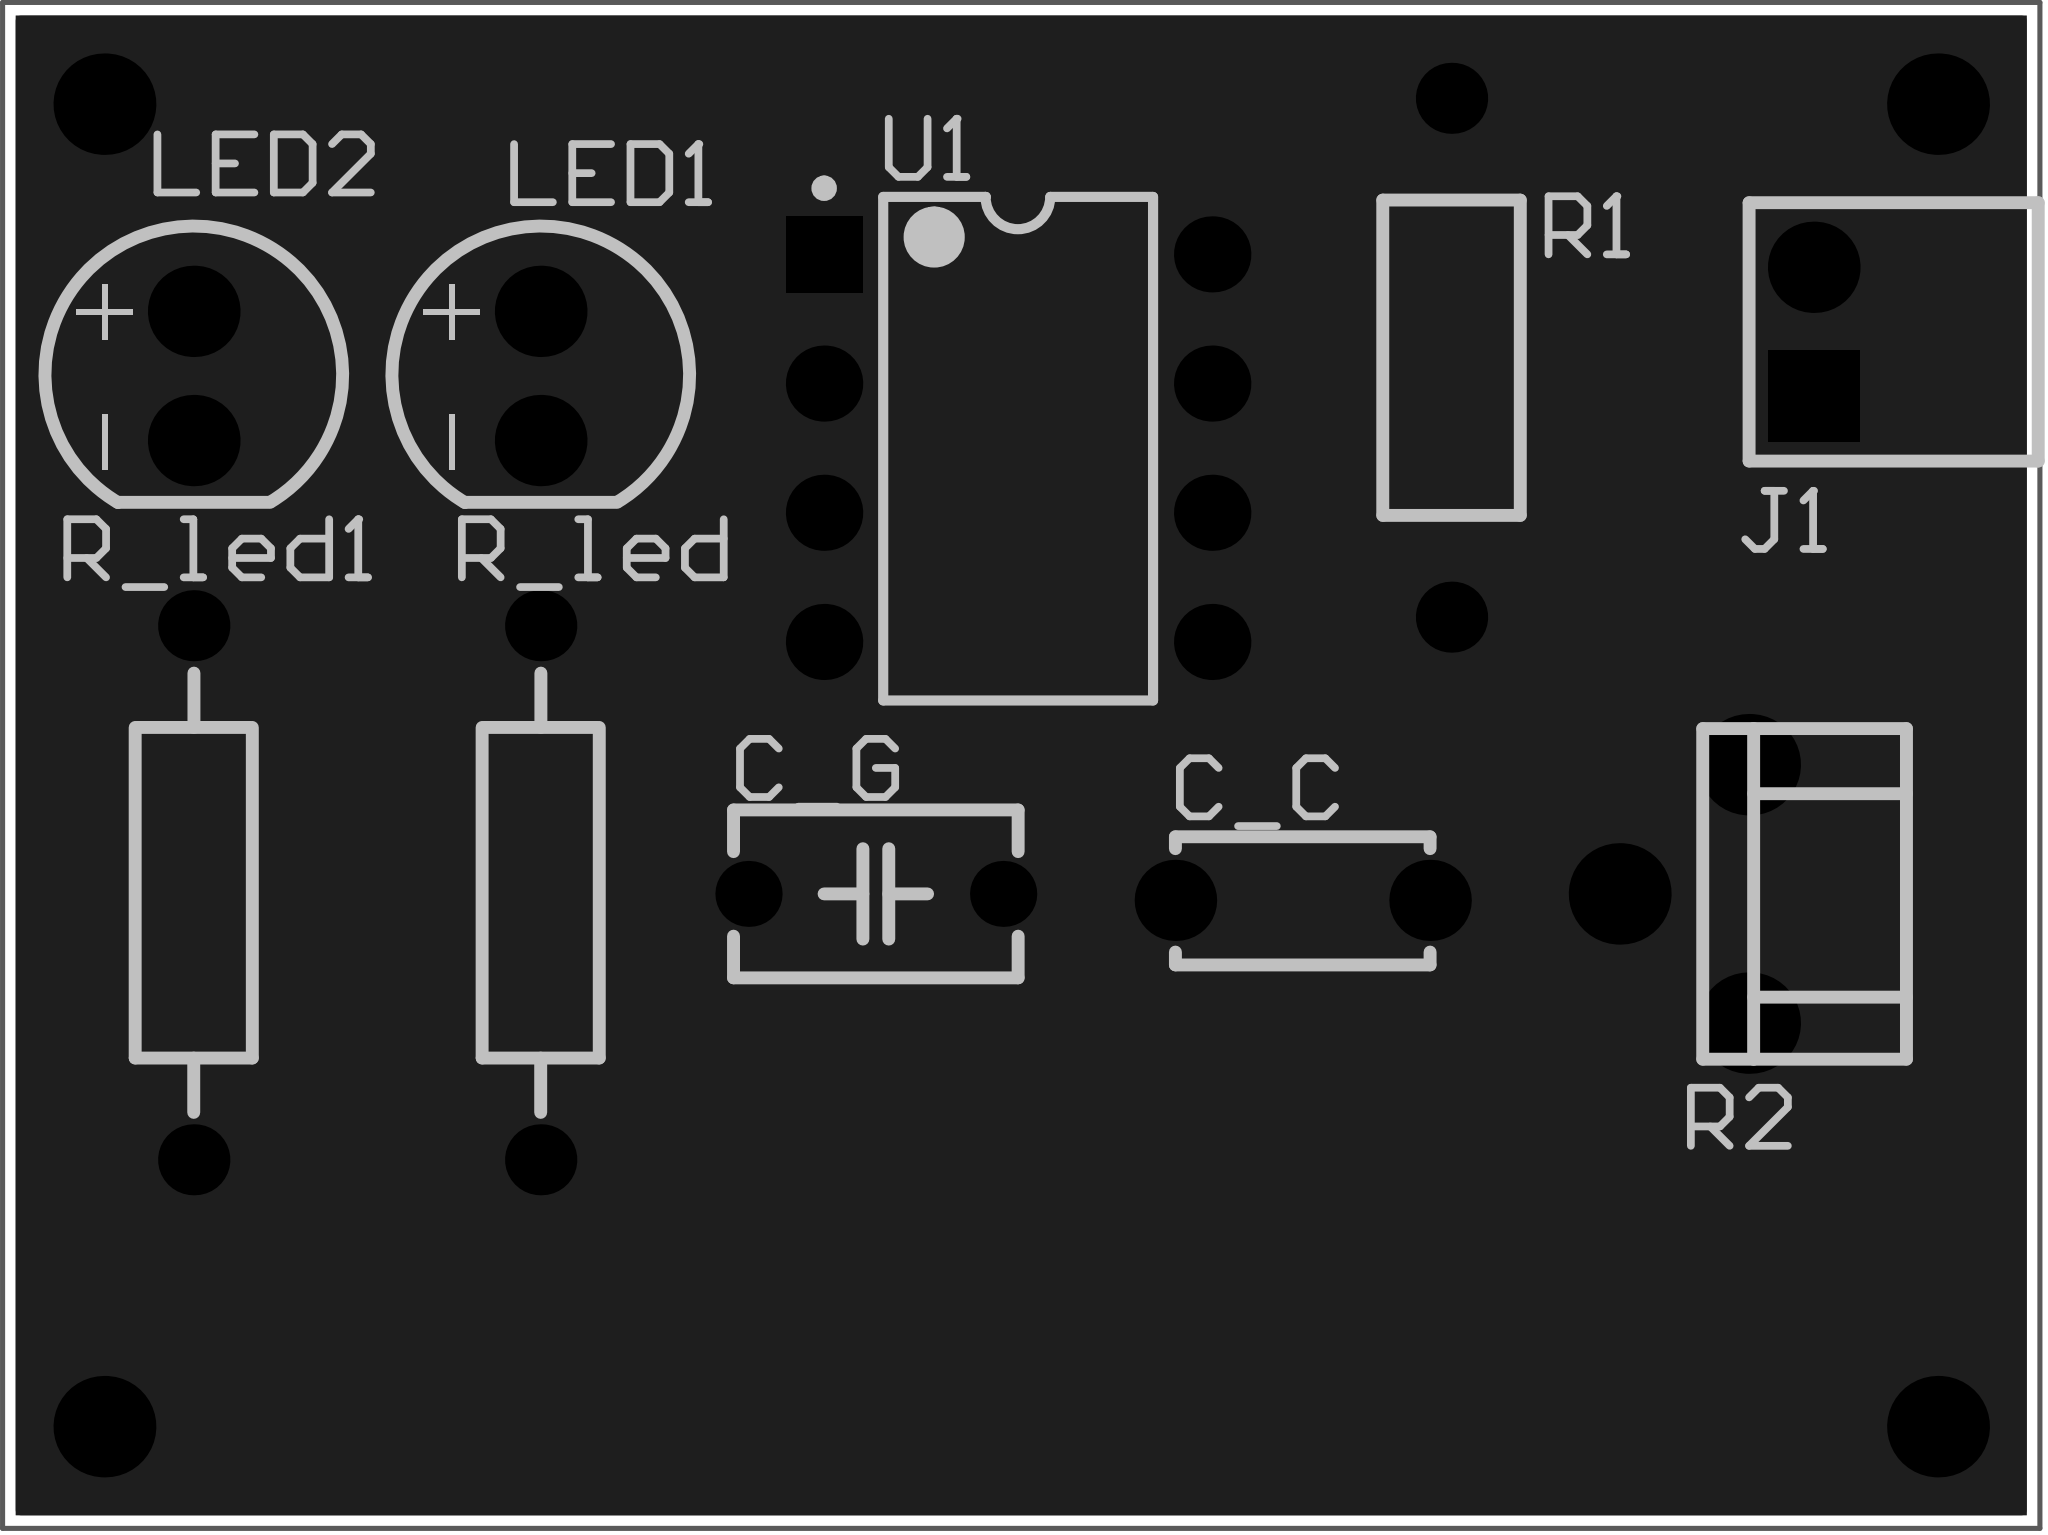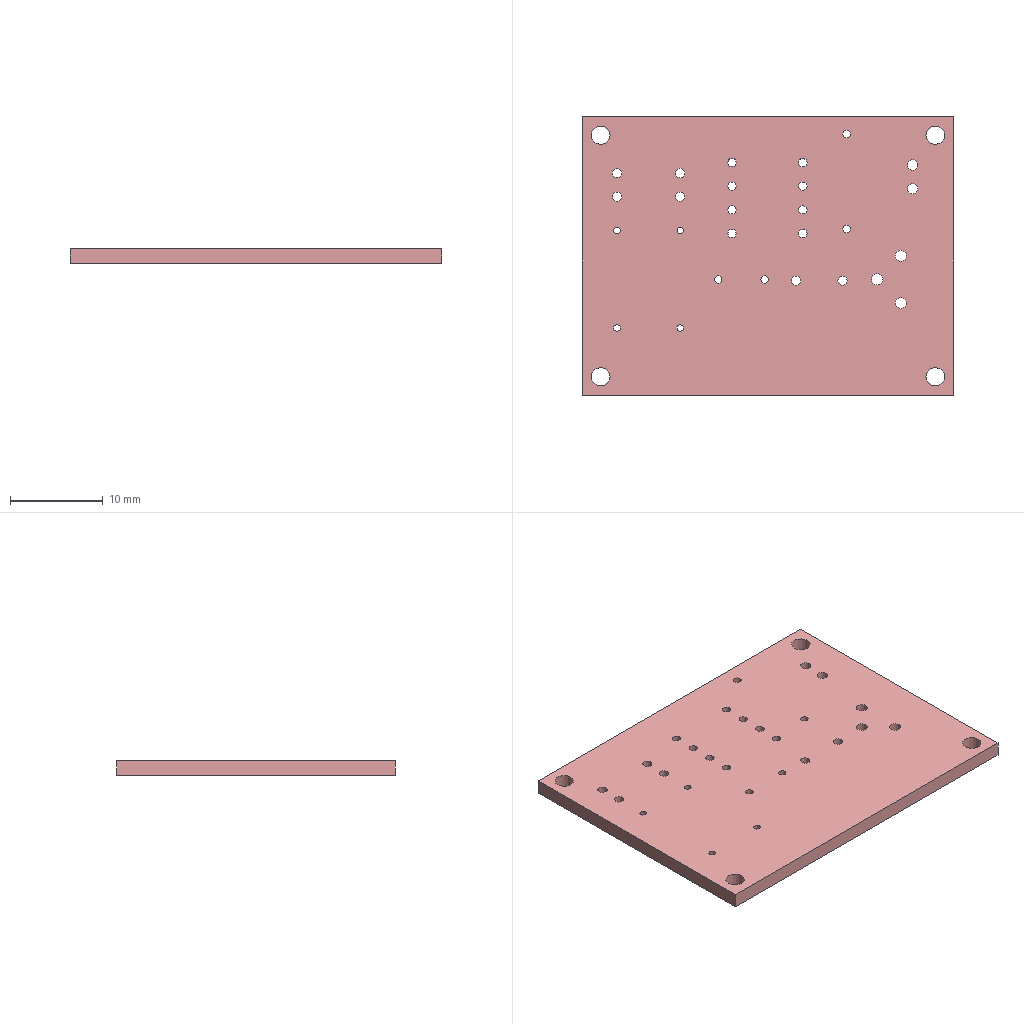Circuit board layout | Altium Designer | box 40 x 30 x 1.6 mm
Layer stack:
# Altium Designer layer stack of  (unit mm; dielectric type: 0 none, 1 core, 2 prepreg, 3 surface material)
index,name,kind,layer,copper_thickness_mm,dielectric_type,dielectric_thickness_mm,dielectric_material,dielectric_constant
0,Top Paste Mask Layer,other,,,,,,
1,Top Silkscreen Layer,other,,,,,,
2,Top Solder Mask Layer,dielectric,,,3,0.01,,3.3
3,Top Layer,copper,Top Layer,0.035,,,,
4,Dielectric1,dielectric,,,3,1.51,FR4,4.5
5,Bottom Layer,copper,Bottom Layer,0.035,,,,
6,Bottom Solder Mask Layer,dielectric,,,3,0.01,,3.3
7,Bottom Silkscreen Layer,other,,,,,,
8,Bottom Paste Mask Layer,other,,,,,,
# drill layer pairs: low layer,high layer
drill_pair,Top Layer,Bottom Layer
Part placement:
Designator,Comment,Layer,Footprint,Center-X(mm),Center-Y(mm),Rotation
J1,,TopLayer,HDR-TH_2P-P2.54-V-M-1,111.76,99.723,90
C_C,100nF,TopLayer,CAP-TH_L5.0-W2.5-P5.00-D1.0,101.727,88.547,0
C_G,10nF,TopLayer,CAP-TH_L5.5-W3.0-P5.00-D0.6,93.345,88.674,0
LED1,XL-502SURD,TopLayer,LED-TH_BD5.9-P2.54-RD_RED,86.765,98.856,90
LED2,XL-502SURD,TopLayer,LED-TH_BD5.9-P2.54-RD_RED,79.953,98.856,90
R1,1kΩ,TopLayer,RES-TH_BD2.7-L6.2-P10.20-D0.4,104.648,99.215,90
R2,1MΩ,TopLayer,RES-ADJ-TH_RM063-103,109.22,88.674,90
R_led,470Ω,TopLayer,RES-TH_BD2.3-L6.5-P10.50-D0.5,86.765,88.697,90
R_led1,470Ω,TopLayer,RES-TH_BD2.3-L6.5-P10.50-D0.5,79.953,88.697,90
U1,NE555P,TopLayer,DIP-8_L9.8-W6.6-P2.54-LS7.6-BL,96.139,97.437,270
Pad and via stacks:
# Altium Designer via and pad stacks of  (unit mm). Each distinct definition once, with the count of objects using it.
# via: kind,start_layer,end_layer,hole_mm,diameter_mm,mode(0 simple;1 top-mid-bottom;2 full stack),diameter_per_layer,count,example_net
# pad: kind,layer,hole_mm,hole_type(0 round;1 square;2 slot),plating,top_size,top_shape(1 round;2 rect;3 octagon;9 rounded rect),mid_size,bottom_size,mode,footprint,size_per_layer,count,example
pad,Multi-Layer,1.1,0,plated,1.8x1.8,1,1.8x1.8,1.8x1.8,0,HDR-TH_2P-P2.54-V-M-1,,1,J1.2
pad,Multi-Layer,1.1,0,plated,1.8x1.8,2,1.8x1.8,1.8x1.8,0,HDR-TH_2P-P2.54-V-M-1,,1,J1.1
pad,Multi-Layer,2,0,plated,2x2,1,2x2,2x2,0,,,4,1
pad,Multi-Layer,1,0,plated,1.6x1.6,1,1.6x1.6,1.6x1.6,0,CAP-TH_L5.0-W2.5-P5.00-D1.0,,2,C_C.1
pad,Multi-Layer,0.8,0,plated,1.3x1.3,1,1.3x1.3,1.3x1.3,0,CAP-TH_L5.5-W3.0-P5.00-D0.6,,2,C_G.2
pad,Multi-Layer,1,0,plated,1.8x1.8,1,1.8x1.8,1.8x1.8,0,LED-TH_BD5.9-P2.54-RD_RED,,4,LED1.2
pad,Multi-Layer,0.8,0,plated,1.4x1.4,1,1.4x1.4,1.4x1.4,0,RES-TH_BD2.7-L6.2-P10.20-D0.4,,2,R1.1
pad,Multi-Layer,1.2,0,plated,2x2,1,2x2,2x2,0,RES-ADJ-TH_RM063-103,,3,R2.1
pad,Multi-Layer,0.7,0,plated,1.4x1.4,1,1.4x1.4,1.4x1.4,0,RES-TH_BD2.3-L6.5-P10.50-D0.5,,4,R_led.1
pad,Multi-Layer,0.9,0,plated,1.5x1.5,2,1.5x1.5,1.5x1.5,0,DIP-8_L9.8-W6.6-P2.54-LS7.6-BL,,1,U1.1
pad,Multi-Layer,0.9,0,plated,1.5x1.5,1,1.5x1.5,1.5x1.5,0,DIP-8_L9.8-W6.6-P2.54-LS7.6-BL,,7,U1.2
Copper pours:
name,layer,net,type(0 solid;1 hatched;2 none)
Top Layer-GND,Top Layer,GND,0
Bottom Layer-GND,Bottom Layer,GND,0
Design rules, without the lines most boards share:
# Altium Designer design rules of  (exported by Altium Designer, unit mm)
# columns: name | kind | enabled | priority | scope1 | scope2 | descriptor | typed fields (field=value)
creepage | 65 | enabled | 1 | All | All | Creepage Distance Constraint =(0mil) (All),(All) |